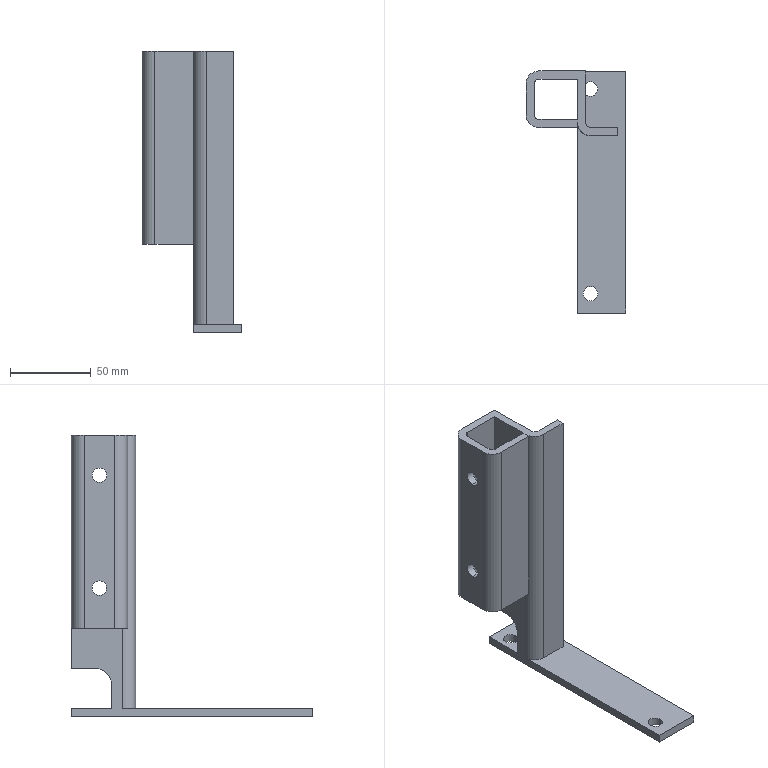Part | SolidWorks | features BaseBody 1 | 1 solid | 40 faces | box 62 x 150 x 175 mm | volume 117135 mm3 | plane 21 | cylinder 19 | commonest cylinder face diameters 9 x12 6 x3 16 x3 20 x1
STEP:
#1=CARTESIAN_POINT('',(0.,-17.5,149.5));
#2=VERTEX_POINT('',#1);
#3=CARTESIAN_POINT('',(0.,-17.5,140.5));
#4=VERTEX_POINT('',#3);
#5=CARTESIAN_POINT('',(0.,-17.5,145.));
#6=DIRECTION('',(1.,0.,0.));
#7=DIRECTION('',(0.,0.,-1.));
#8=AXIS2_PLACEMENT_3D('',#5,#6,#7);
#9=CIRCLE('',#8,4.5);
#10=EDGE_CURVE('',#2,#4,#9,.T.);
#11=ORIENTED_EDGE('',*,*,#10,.F.);
#12=CARTESIAN_POINT('',(5.,-17.5,149.5));
#13=VERTEX_POINT('',#12);
#14=CARTESIAN_POINT('',(0.,-17.5,149.5));
#15=DIRECTION('',(1.,0.,0.));
#16=VECTOR('',#15,1000.);
#17=LINE('',#14,#16);
#18=EDGE_CURVE('',#2,#13,#17,.T.);
#19=ORIENTED_EDGE('',*,*,#18,.T.);
#20=CARTESIAN_POINT('',(5.,-17.5,140.5));
#21=VERTEX_POINT('',#20);
#22=CARTESIAN_POINT('',(5.,-17.5,145.));
#23=DIRECTION('',(-1.,0.,0.));
#24=DIRECTION('',(0.,0.,-1.));
#25=AXIS2_PLACEMENT_3D('',#22,#23,#24);
#26=CIRCLE('',#25,4.5);
#27=EDGE_CURVE('',#21,#13,#26,.T.);
#28=ORIENTED_EDGE('',*,*,#27,.F.);
#29=CARTESIAN_POINT('',(0.,-17.5,140.5));
#30=DIRECTION('',(1.,0.,0.));
#31=VECTOR('',#30,1000.);
#32=LINE('',#29,#31);
#33=EDGE_CURVE('',#4,#21,#32,.T.);
#34=ORIENTED_EDGE('',*,*,#33,.F.);
#35=EDGE_LOOP('',(#11,#19,#28,#34));
#36=FACE_OUTER_BOUND('',#35,.T.);
#37=CARTESIAN_POINT('',(0.,-17.5,145.));
#38=DIRECTION('',(1.,0.,0.));
#39=DIRECTION('',(0.,0.,-1.));
#40=AXIS2_PLACEMENT_3D('',#37,#38,#39);
#41=CYLINDRICAL_SURFACE('',#40,4.5);
#42=ADVANCED_FACE('',(#36),#41,.F.);
#43=CARTESIAN_POINT('',(0.,-17.5,79.5));
#44=VERTEX_POINT('',#43);
#45=CARTESIAN_POINT('',(0.,-17.5,70.5));
#46=VERTEX_POINT('',#45);
#47=CARTESIAN_POINT('',(0.,-17.5,75.));
#48=DIRECTION('',(1.,0.,0.));
#49=DIRECTION('',(0.,0.,-1.));
#50=AXIS2_PLACEMENT_3D('',#47,#48,#49);
#51=CIRCLE('',#50,4.5);
#52=EDGE_CURVE('',#44,#46,#51,.T.);
#53=ORIENTED_EDGE('',*,*,#52,.F.);
#54=CARTESIAN_POINT('',(5.,-17.5,79.5));
#55=VERTEX_POINT('',#54);
#56=CARTESIAN_POINT('',(0.,-17.5,79.5));
#57=DIRECTION('',(1.,0.,0.));
#58=VECTOR('',#57,1000.);
#59=LINE('',#56,#58);
#60=EDGE_CURVE('',#44,#55,#59,.T.);
#61=ORIENTED_EDGE('',*,*,#60,.T.);
#62=CARTESIAN_POINT('',(5.,-17.5,70.5));
#63=VERTEX_POINT('',#62);
#64=CARTESIAN_POINT('',(5.,-17.5,75.));
#65=DIRECTION('',(-1.,0.,0.));
#66=DIRECTION('',(0.,0.,-1.));
#67=AXIS2_PLACEMENT_3D('',#64,#65,#66);
#68=CIRCLE('',#67,4.5);
#69=EDGE_CURVE('',#63,#55,#68,.T.);
#70=ORIENTED_EDGE('',*,*,#69,.F.);
#71=CARTESIAN_POINT('',(0.,-17.5,70.5));
#72=DIRECTION('',(1.,0.,0.));
#73=VECTOR('',#72,1000.);
#74=LINE('',#71,#73);
#75=EDGE_CURVE('',#46,#63,#74,.T.);
#76=ORIENTED_EDGE('',*,*,#75,.F.);
#77=EDGE_LOOP('',(#53,#61,#70,#76));
#78=FACE_OUTER_BOUND('',#77,.T.);
#79=CARTESIAN_POINT('',(0.,-17.5,75.));
#80=DIRECTION('',(1.,0.,0.));
#81=DIRECTION('',(0.,0.,-1.));
#82=AXIS2_PLACEMENT_3D('',#79,#80,#81);
#83=CYLINDRICAL_SURFACE('',#82,4.5);
#84=ADVANCED_FACE('',(#78),#83,.F.);
#85=CARTESIAN_POINT('',(3.5,-11.,-5.));
#86=VERTEX_POINT('',#85);
#87=CARTESIAN_POINT('',(12.5,-11.,-5.));
#88=VERTEX_POINT('',#87);
#89=CARTESIAN_POINT('',(8.,-11.,-5.));
#90=DIRECTION('',(0.,0.,1.));
#91=DIRECTION('',(1.,0.,0.));
#92=AXIS2_PLACEMENT_3D('',#89,#90,#91);
#93=CIRCLE('',#92,4.5);
#94=EDGE_CURVE('',#86,#88,#93,.T.);
#95=ORIENTED_EDGE('',*,*,#94,.F.);
#96=CARTESIAN_POINT('',(3.5,-11.,0.));
#97=VERTEX_POINT('',#96);
#98=CARTESIAN_POINT('',(3.5,-11.,-5.));
#99=DIRECTION('',(0.,0.,1.));
#100=VECTOR('',#99,1000.);
#101=LINE('',#98,#100);
#102=EDGE_CURVE('',#86,#97,#101,.T.);
#103=ORIENTED_EDGE('',*,*,#102,.T.);
#104=CARTESIAN_POINT('',(12.5,-11.,0.));
#105=VERTEX_POINT('',#104);
#106=CARTESIAN_POINT('',(8.,-11.,0.));
#107=DIRECTION('',(0.,0.,-1.));
#108=DIRECTION('',(1.,0.,0.));
#109=AXIS2_PLACEMENT_3D('',#106,#107,#108);
#110=CIRCLE('',#109,4.5);
#111=EDGE_CURVE('',#105,#97,#110,.T.);
#112=ORIENTED_EDGE('',*,*,#111,.F.);
#113=CARTESIAN_POINT('',(12.5,-11.,-5.));
#114=DIRECTION('',(0.,0.,1.));
#115=VECTOR('',#114,1000.);
#116=LINE('',#113,#115);
#117=EDGE_CURVE('',#88,#105,#116,.T.);
#118=ORIENTED_EDGE('',*,*,#117,.F.);
#119=EDGE_LOOP('',(#95,#103,#112,#118));
#120=FACE_OUTER_BOUND('',#119,.T.);
#121=CARTESIAN_POINT('',(8.,-11.,-5.));
#122=DIRECTION('',(0.,0.,1.));
#123=DIRECTION('',(1.,0.,0.));
#124=AXIS2_PLACEMENT_3D('',#121,#122,#123);
#125=CYLINDRICAL_SURFACE('',#124,4.5);
#126=ADVANCED_FACE('',(#120),#125,.F.);
#127=CARTESIAN_POINT('',(3.5,-138.,-5.));
#128=VERTEX_POINT('',#127);
#129=CARTESIAN_POINT('',(12.5,-138.,-5.));
#130=VERTEX_POINT('',#129);
#131=CARTESIAN_POINT('',(8.,-138.,-5.));
#132=DIRECTION('',(0.,0.,1.));
#133=DIRECTION('',(1.,0.,0.));
#134=AXIS2_PLACEMENT_3D('',#131,#132,#133);
#135=CIRCLE('',#134,4.5);
#136=EDGE_CURVE('',#128,#130,#135,.T.);
#137=ORIENTED_EDGE('',*,*,#136,.F.);
#138=CARTESIAN_POINT('',(3.5,-138.,0.));
#139=VERTEX_POINT('',#138);
#140=CARTESIAN_POINT('',(3.5,-138.,-5.));
#141=DIRECTION('',(0.,0.,1.));
#142=VECTOR('',#141,1000.);
#143=LINE('',#140,#142);
#144=EDGE_CURVE('',#128,#139,#143,.T.);
#145=ORIENTED_EDGE('',*,*,#144,.T.);
#146=CARTESIAN_POINT('',(12.5,-138.,0.));
#147=VERTEX_POINT('',#146);
#148=CARTESIAN_POINT('',(8.,-138.,0.));
#149=DIRECTION('',(0.,0.,-1.));
#150=DIRECTION('',(1.,0.,0.));
#151=AXIS2_PLACEMENT_3D('',#148,#149,#150);
#152=CIRCLE('',#151,4.5);
#153=EDGE_CURVE('',#147,#139,#152,.T.);
#154=ORIENTED_EDGE('',*,*,#153,.F.);
#155=CARTESIAN_POINT('',(12.5,-138.,-5.));
#156=DIRECTION('',(0.,0.,1.));
#157=VECTOR('',#156,1000.);
#158=LINE('',#155,#157);
#159=EDGE_CURVE('',#130,#147,#158,.T.);
#160=ORIENTED_EDGE('',*,*,#159,.F.);
#161=EDGE_LOOP('',(#137,#145,#154,#160));
#162=FACE_OUTER_BOUND('',#161,.T.);
#163=CARTESIAN_POINT('',(8.,-138.,-5.));
#164=DIRECTION('',(0.,0.,1.));
#165=DIRECTION('',(1.,0.,0.));
#166=AXIS2_PLACEMENT_3D('',#163,#164,#165);
#167=CYLINDRICAL_SURFACE('',#166,4.5);
#168=ADVANCED_FACE('',(#162),#167,.F.);
#169=CARTESIAN_POINT('',(-27.,-17.5,140.5));
#170=VERTEX_POINT('',#169);
#171=CARTESIAN_POINT('',(-27.,-17.5,149.5));
#172=VERTEX_POINT('',#171);
#173=CARTESIAN_POINT('',(-27.,-17.5,145.));
#174=DIRECTION('',(-1.,0.,0.));
#175=DIRECTION('',(0.,0.,1.));
#176=AXIS2_PLACEMENT_3D('',#173,#174,#175);
#177=CIRCLE('',#176,4.5);
#178=EDGE_CURVE('',#170,#172,#177,.T.);
#179=ORIENTED_EDGE('',*,*,#178,.F.);
#180=CARTESIAN_POINT('',(-32.,-17.5,140.5));
#181=VERTEX_POINT('',#180);
#182=CARTESIAN_POINT('',(-27.,-17.5,140.5));
#183=DIRECTION('',(-1.,0.,0.));
#184=VECTOR('',#183,1000.);
#185=LINE('',#182,#184);
#186=EDGE_CURVE('',#170,#181,#185,.T.);
#187=ORIENTED_EDGE('',*,*,#186,.T.);
#188=CARTESIAN_POINT('',(-32.,-17.5,149.5));
#189=VERTEX_POINT('',#188);
#190=CARTESIAN_POINT('',(-32.,-17.5,145.));
#191=DIRECTION('',(-1.,0.,0.));
#192=DIRECTION('',(0.,0.,1.));
#193=AXIS2_PLACEMENT_3D('',#190,#191,#192);
#194=CIRCLE('',#193,4.5);
#195=EDGE_CURVE('',#181,#189,#194,.T.);
#196=ORIENTED_EDGE('',*,*,#195,.T.);
#197=CARTESIAN_POINT('',(-27.,-17.5,149.5));
#198=DIRECTION('',(-1.,0.,0.));
#199=VECTOR('',#198,1000.);
#200=LINE('',#197,#199);
#201=EDGE_CURVE('',#172,#189,#200,.T.);
#202=ORIENTED_EDGE('',*,*,#201,.F.);
#203=EDGE_LOOP('',(#179,#187,#196,#202));
#204=FACE_OUTER_BOUND('',#203,.T.);
#205=CARTESIAN_POINT('',(-27.,-17.5,145.));
#206=DIRECTION('',(-1.,0.,0.));
#207=DIRECTION('',(0.,0.,1.));
#208=AXIS2_PLACEMENT_3D('',#205,#206,#207);
#209=CYLINDRICAL_SURFACE('',#208,4.5);
#210=ADVANCED_FACE('',(#204),#209,.F.);
#211=CARTESIAN_POINT('',(-27.,-17.5,70.5));
#212=VERTEX_POINT('',#211);
#213=CARTESIAN_POINT('',(-27.,-17.5,79.5));
#214=VERTEX_POINT('',#213);
#215=CARTESIAN_POINT('',(-27.,-17.5,75.));
#216=DIRECTION('',(-1.,0.,0.));
#217=DIRECTION('',(0.,0.,1.));
#218=AXIS2_PLACEMENT_3D('',#215,#216,#217);
#219=CIRCLE('',#218,4.5);
#220=EDGE_CURVE('',#212,#214,#219,.T.);
#221=ORIENTED_EDGE('',*,*,#220,.F.);
#222=CARTESIAN_POINT('',(-32.,-17.5,70.5));
#223=VERTEX_POINT('',#222);
#224=CARTESIAN_POINT('',(-27.,-17.5,70.5));
#225=DIRECTION('',(-1.,0.,0.));
#226=VECTOR('',#225,1000.);
#227=LINE('',#224,#226);
#228=EDGE_CURVE('',#212,#223,#227,.T.);
#229=ORIENTED_EDGE('',*,*,#228,.T.);
#230=CARTESIAN_POINT('',(-32.,-17.5,79.5));
#231=VERTEX_POINT('',#230);
#232=CARTESIAN_POINT('',(-32.,-17.5,75.));
#233=DIRECTION('',(-1.,0.,0.));
#234=DIRECTION('',(0.,0.,1.));
#235=AXIS2_PLACEMENT_3D('',#232,#233,#234);
#236=CIRCLE('',#235,4.5);
#237=EDGE_CURVE('',#223,#231,#236,.T.);
#238=ORIENTED_EDGE('',*,*,#237,.T.);
#239=CARTESIAN_POINT('',(-27.,-17.5,79.5));
#240=DIRECTION('',(-1.,0.,0.));
#241=VECTOR('',#240,1000.);
#242=LINE('',#239,#241);
#243=EDGE_CURVE('',#214,#231,#242,.T.);
#244=ORIENTED_EDGE('',*,*,#243,.F.);
#245=EDGE_LOOP('',(#221,#229,#238,#244));
#246=FACE_OUTER_BOUND('',#245,.T.);
#247=CARTESIAN_POINT('',(-27.,-17.5,75.));
#248=DIRECTION('',(-1.,0.,0.));
#249=DIRECTION('',(0.,0.,1.));
#250=AXIS2_PLACEMENT_3D('',#247,#248,#249);
#251=CYLINDRICAL_SURFACE('',#250,4.5);
#252=ADVANCED_FACE('',(#246),#251,.F.);
#253=ORIENTED_EDGE('',*,*,#27,.T.);
#254=CARTESIAN_POINT('',(5.,-17.5,145.));
#255=DIRECTION('',(-1.,0.,0.));
#256=DIRECTION('',(0.,0.,-1.));
#257=AXIS2_PLACEMENT_3D('',#254,#255,#256);
#258=CIRCLE('',#257,4.5);
#259=EDGE_CURVE('',#13,#21,#258,.T.);
#260=ORIENTED_EDGE('',*,*,#259,.T.);
#261=EDGE_LOOP('',(#253,#260));
#262=FACE_BOUND('',#261,.T.);
#263=ORIENTED_EDGE('',*,*,#69,.T.);
#264=CARTESIAN_POINT('',(5.,-17.5,75.));
#265=DIRECTION('',(-1.,0.,0.));
#266=DIRECTION('',(0.,0.,-1.));
#267=AXIS2_PLACEMENT_3D('',#264,#265,#266);
#268=CIRCLE('',#267,4.5);
#269=EDGE_CURVE('',#55,#63,#268,.T.);
#270=ORIENTED_EDGE('',*,*,#269,.T.);
#271=EDGE_LOOP('',(#263,#270));
#272=FACE_BOUND('',#271,.T.);
#273=CARTESIAN_POINT('',(5.,0.,170.));
#274=VERTEX_POINT('',#273);
#275=CARTESIAN_POINT('',(5.,-32.,170.));
#276=VERTEX_POINT('',#275);
#277=CARTESIAN_POINT('',(5.,-16.,170.));
#278=DIRECTION('',(0.,-1.,0.));
#279=VECTOR('',#278,1000.);
#280=LINE('',#277,#279);
#281=EDGE_CURVE('',#274,#276,#280,.T.);
#282=ORIENTED_EDGE('',*,*,#281,.T.);
#283=CARTESIAN_POINT('',(5.,-32.,0.));
#284=VERTEX_POINT('',#283);
#285=CARTESIAN_POINT('',(5.,-32.,85.));
#286=DIRECTION('',(0.,0.,-1.));
#287=VECTOR('',#286,1000.);
#288=LINE('',#285,#287);
#289=EDGE_CURVE('',#276,#284,#288,.T.);
#290=ORIENTED_EDGE('',*,*,#289,.T.);
#291=CARTESIAN_POINT('',(5.,-25.,0.));
#292=VERTEX_POINT('',#291);
#293=CARTESIAN_POINT('',(5.,-16.,0.));
#294=DIRECTION('',(0.,1.,0.));
#295=VECTOR('',#294,1000.);
#296=LINE('',#293,#295);
#297=EDGE_CURVE('',#284,#292,#296,.T.);
#298=ORIENTED_EDGE('',*,*,#297,.T.);
#299=CARTESIAN_POINT('',(5.,-25.,15.));
#300=VERTEX_POINT('',#299);
#301=CARTESIAN_POINT('',(5.,-25.,85.));
#302=DIRECTION('',(0.,0.,1.));
#303=VECTOR('',#302,1000.);
#304=LINE('',#301,#303);
#305=EDGE_CURVE('',#292,#300,#304,.T.);
#306=ORIENTED_EDGE('',*,*,#305,.T.);
#307=CARTESIAN_POINT('',(5.,-15.,25.));
#308=VERTEX_POINT('',#307);
#309=CARTESIAN_POINT('',(5.,-15.,15.));
#310=DIRECTION('',(-1.,0.,0.));
#311=DIRECTION('',(0.,0.,-1.));
#312=AXIS2_PLACEMENT_3D('',#309,#310,#311);
#313=CIRCLE('',#312,10.);
#314=EDGE_CURVE('',#300,#308,#313,.T.);
#315=ORIENTED_EDGE('',*,*,#314,.T.);
#316=CARTESIAN_POINT('',(5.,0.,25.));
#317=VERTEX_POINT('',#316);
#318=CARTESIAN_POINT('',(5.,-16.,25.));
#319=DIRECTION('',(0.,1.,0.));
#320=VECTOR('',#319,1000.);
#321=LINE('',#318,#320);
#322=EDGE_CURVE('',#308,#317,#321,.T.);
#323=ORIENTED_EDGE('',*,*,#322,.T.);
#324=CARTESIAN_POINT('',(5.,0.,85.));
#325=DIRECTION('',(0.,0.,1.));
#326=VECTOR('',#325,1000.);
#327=LINE('',#324,#326);
#328=EDGE_CURVE('',#317,#274,#327,.T.);
#329=ORIENTED_EDGE('',*,*,#328,.T.);
#330=EDGE_LOOP('',(#282,#290,#298,#306,#315,#323,#329));
#331=FACE_OUTER_BOUND('',#330,.T.);
#332=CARTESIAN_POINT('',(5.,-16.,85.));
#333=DIRECTION('',(1.,0.,0.));
#334=DIRECTION('',(0.,0.,-1.));
#335=AXIS2_PLACEMENT_3D('',#332,#333,#334);
#336=PLANE('',#335);
#337=ADVANCED_FACE('',(#262,#272,#331),#336,.T.);
#338=ORIENTED_EDGE('',*,*,#18,.F.);
#339=CARTESIAN_POINT('',(0.,-17.5,145.));
#340=DIRECTION('',(1.,0.,0.));
#341=DIRECTION('',(0.,0.,-1.));
#342=AXIS2_PLACEMENT_3D('',#339,#340,#341);
#343=CIRCLE('',#342,4.5);
#344=EDGE_CURVE('',#4,#2,#343,.T.);
#345=ORIENTED_EDGE('',*,*,#344,.F.);
#346=ORIENTED_EDGE('',*,*,#33,.T.);
#347=ORIENTED_EDGE('',*,*,#259,.F.);
#348=EDGE_LOOP('',(#338,#345,#346,#347));
#349=FACE_OUTER_BOUND('',#348,.T.);
#350=CARTESIAN_POINT('',(0.,-17.5,145.));
#351=DIRECTION('',(1.,0.,0.));
#352=DIRECTION('',(0.,0.,-1.));
#353=AXIS2_PLACEMENT_3D('',#350,#351,#352);
#354=CYLINDRICAL_SURFACE('',#353,4.5);
#355=ADVANCED_FACE('',(#349),#354,.F.);
#356=ORIENTED_EDGE('',*,*,#60,.F.);
#357=CARTESIAN_POINT('',(0.,-17.5,75.));
#358=DIRECTION('',(1.,0.,0.));
#359=DIRECTION('',(0.,0.,-1.));
#360=AXIS2_PLACEMENT_3D('',#357,#358,#359);
#361=CIRCLE('',#360,4.5);
#362=EDGE_CURVE('',#46,#44,#361,.T.);
#363=ORIENTED_EDGE('',*,*,#362,.F.);
#364=ORIENTED_EDGE('',*,*,#75,.T.);
#365=ORIENTED_EDGE('',*,*,#269,.F.);
#366=EDGE_LOOP('',(#356,#363,#364,#365));
#367=FACE_OUTER_BOUND('',#366,.T.);
#368=CARTESIAN_POINT('',(0.,-17.5,75.));
#369=DIRECTION('',(1.,0.,0.));
#370=DIRECTION('',(0.,0.,-1.));
#371=AXIS2_PLACEMENT_3D('',#368,#369,#370);
#372=CYLINDRICAL_SURFACE('',#371,4.5);
#373=ADVANCED_FACE('',(#367),#372,.F.);
#374=CARTESIAN_POINT('',(8.,-35.,170.));
#375=VERTEX_POINT('',#374);
#376=CARTESIAN_POINT('',(8.,-32.,170.));
#377=DIRECTION('',(0.,0.,-1.));
#378=DIRECTION('',(-1.,0.,0.));
#379=AXIS2_PLACEMENT_3D('',#376,#377,#378);
#380=CIRCLE('',#379,3.);
#381=EDGE_CURVE('',#375,#276,#380,.T.);
#382=ORIENTED_EDGE('',*,*,#381,.F.);
#383=CARTESIAN_POINT('',(8.,-35.,0.));
#384=VERTEX_POINT('',#383);
#385=CARTESIAN_POINT('',(8.,-35.,170.));
#386=DIRECTION('',(0.,0.,1.));
#387=VECTOR('',#386,1000.);
#388=LINE('',#385,#387);
#389=EDGE_CURVE('',#384,#375,#388,.T.);
#390=ORIENTED_EDGE('',*,*,#389,.F.);
#391=CARTESIAN_POINT('',(8.,-32.,0.));
#392=DIRECTION('',(0.,0.,1.));
#393=DIRECTION('',(-1.,0.,0.));
#394=AXIS2_PLACEMENT_3D('',#391,#392,#393);
#395=CIRCLE('',#394,3.);
#396=EDGE_CURVE('',#284,#384,#395,.T.);
#397=ORIENTED_EDGE('',*,*,#396,.F.);
#398=ORIENTED_EDGE('',*,*,#289,.F.);
#399=EDGE_LOOP('',(#382,#390,#397,#398));
#400=FACE_OUTER_BOUND('',#399,.T.);
#401=CARTESIAN_POINT('',(8.,-32.,170.));
#402=DIRECTION('',(0.,0.,-1.));
#403=DIRECTION('',(-1.,0.,0.));
#404=AXIS2_PLACEMENT_3D('',#401,#402,#403);
#405=CYLINDRICAL_SURFACE('',#404,3.);
#406=ADVANCED_FACE('',(#400),#405,.F.);
#407=CARTESIAN_POINT('',(-24.,-5.,170.));
#408=VERTEX_POINT('',#407);
#409=CARTESIAN_POINT('',(0.,-5.,170.));
#410=VERTEX_POINT('',#409);
#411=CARTESIAN_POINT('',(12.5,-5.,170.));
#412=DIRECTION('',(1.,0.,0.));
#413=VECTOR('',#412,1000.);
#414=LINE('',#411,#413);
#415=EDGE_CURVE('',#408,#410,#414,.T.);
#416=ORIENTED_EDGE('',*,*,#415,.T.);
#417=CARTESIAN_POINT('',(0.,-30.,170.));
#418=VERTEX_POINT('',#417);
#419=CARTESIAN_POINT('',(0.,-20.,170.));
#420=DIRECTION('',(0.,-1.,0.));
#421=VECTOR('',#420,1000.);
#422=LINE('',#419,#421);
#423=EDGE_CURVE('',#410,#418,#422,.T.);
#424=ORIENTED_EDGE('',*,*,#423,.T.);
#425=CARTESIAN_POINT('',(-24.,-30.,170.));
#426=VERTEX_POINT('',#425);
#427=CARTESIAN_POINT('',(12.5,-30.,170.));
#428=DIRECTION('',(-1.,0.,0.));
#429=VECTOR('',#428,1000.);
#430=LINE('',#427,#429);
#431=EDGE_CURVE('',#418,#426,#430,.T.);
#432=ORIENTED_EDGE('',*,*,#431,.T.);
#433=CARTESIAN_POINT('',(-27.,-27.,170.));
#434=VERTEX_POINT('',#433);
#435=CARTESIAN_POINT('',(-24.,-27.,170.));
#436=DIRECTION('',(0.,0.,-1.));
#437=DIRECTION('',(1.,0.,0.));
#438=AXIS2_PLACEMENT_3D('',#435,#436,#437);
#439=CIRCLE('',#438,3.);
#440=EDGE_CURVE('',#426,#434,#439,.T.);
#441=ORIENTED_EDGE('',*,*,#440,.T.);
#442=CARTESIAN_POINT('',(-27.,-8.,170.));
#443=VERTEX_POINT('',#442);
#444=CARTESIAN_POINT('',(-27.,-20.,170.));
#445=DIRECTION('',(0.,1.,0.));
#446=VECTOR('',#445,1000.);
#447=LINE('',#444,#446);
#448=EDGE_CURVE('',#434,#443,#447,.T.);
#449=ORIENTED_EDGE('',*,*,#448,.T.);
#450=CARTESIAN_POINT('',(-24.,-8.,170.));
#451=DIRECTION('',(0.,0.,-1.));
#452=DIRECTION('',(1.,0.,0.));
#453=AXIS2_PLACEMENT_3D('',#450,#451,#452);
#454=CIRCLE('',#453,3.);
#455=EDGE_CURVE('',#443,#408,#454,.T.);
#456=ORIENTED_EDGE('',*,*,#455,.T.);
#457=EDGE_LOOP('',(#416,#424,#432,#441,#449,#456));
#458=FACE_BOUND('',#457,.T.);
#459=CARTESIAN_POINT('',(0.,-35.,170.));
#460=VERTEX_POINT('',#459);
#461=CARTESIAN_POINT('',(0.,-32.,170.));
#462=VERTEX_POINT('',#461);
#463=CARTESIAN_POINT('',(0.,-20.,170.));
#464=DIRECTION('',(0.,1.,0.));
#465=VECTOR('',#464,1000.);
#466=LINE('',#463,#465);
#467=EDGE_CURVE('',#460,#462,#466,.T.);
#468=ORIENTED_EDGE('',*,*,#467,.T.);
#469=CARTESIAN_POINT('',(8.,-40.,170.));
#470=VERTEX_POINT('',#469);
#471=CARTESIAN_POINT('',(8.,-32.,170.));
#472=DIRECTION('',(0.,0.,1.));
#473=DIRECTION('',(-1.,0.,0.));
#474=AXIS2_PLACEMENT_3D('',#471,#472,#473);
#475=CIRCLE('',#474,8.);
#476=EDGE_CURVE('',#462,#470,#475,.T.);
#477=ORIENTED_EDGE('',*,*,#476,.T.);
#478=CARTESIAN_POINT('',(25.,-40.,170.));
#479=VERTEX_POINT('',#478);
#480=CARTESIAN_POINT('',(12.5,-40.,170.));
#481=DIRECTION('',(1.,0.,0.));
#482=VECTOR('',#481,1000.);
#483=LINE('',#480,#482);
#484=EDGE_CURVE('',#470,#479,#483,.T.);
#485=ORIENTED_EDGE('',*,*,#484,.T.);
#486=CARTESIAN_POINT('',(25.,-35.,170.));
#487=VERTEX_POINT('',#486);
#488=CARTESIAN_POINT('',(25.,-20.,170.));
#489=DIRECTION('',(0.,1.,0.));
#490=VECTOR('',#489,1000.);
#491=LINE('',#488,#490);
#492=EDGE_CURVE('',#479,#487,#491,.T.);
#493=ORIENTED_EDGE('',*,*,#492,.T.);
#494=CARTESIAN_POINT('',(12.5,-35.,170.));
#495=DIRECTION('',(-1.,0.,0.));
#496=VECTOR('',#495,1000.);
#497=LINE('',#494,#496);
#498=EDGE_CURVE('',#487,#375,#497,.T.);
#499=ORIENTED_EDGE('',*,*,#498,.T.);
#500=ORIENTED_EDGE('',*,*,#381,.T.);
#501=ORIENTED_EDGE('',*,*,#281,.F.);
#502=CARTESIAN_POINT('',(-24.,0.,170.));
#503=VERTEX_POINT('',#502);
#504=CARTESIAN_POINT('',(12.5,0.,170.));
#505=DIRECTION('',(-1.,0.,0.));
#506=VECTOR('',#505,1000.);
#507=LINE('',#504,#506);
#508=EDGE_CURVE('',#274,#503,#507,.T.);
#509=ORIENTED_EDGE('',*,*,#508,.T.);
#510=CARTESIAN_POINT('',(-32.,-8.,170.));
#511=VERTEX_POINT('',#510);
#512=CARTESIAN_POINT('',(-24.,-8.,170.));
#513=DIRECTION('',(0.,0.,1.));
#514=DIRECTION('',(1.,0.,0.));
#515=AXIS2_PLACEMENT_3D('',#512,#513,#514);
#516=CIRCLE('',#515,8.);
#517=EDGE_CURVE('',#503,#511,#516,.T.);
#518=ORIENTED_EDGE('',*,*,#517,.T.);
#519=CARTESIAN_POINT('',(-32.,-27.,170.));
#520=VERTEX_POINT('',#519);
#521=CARTESIAN_POINT('',(-32.,-20.,170.));
#522=DIRECTION('',(0.,-1.,0.));
#523=VECTOR('',#522,1000.);
#524=LINE('',#521,#523);
#525=EDGE_CURVE('',#511,#520,#524,.T.);
#526=ORIENTED_EDGE('',*,*,#525,.T.);
#527=CARTESIAN_POINT('',(-24.,-35.,170.));
#528=VERTEX_POINT('',#527);
#529=CARTESIAN_POINT('',(-24.,-27.,170.));
#530=DIRECTION('',(0.,0.,1.));
#531=DIRECTION('',(1.,0.,0.));
#532=AXIS2_PLACEMENT_3D('',#529,#530,#531);
#533=CIRCLE('',#532,8.);
#534=EDGE_CURVE('',#520,#528,#533,.T.);
#535=ORIENTED_EDGE('',*,*,#534,.T.);
#536=CARTESIAN_POINT('',(12.5,-35.,170.));
#537=DIRECTION('',(1.,0.,0.));
#538=VECTOR('',#537,1000.);
#539=LINE('',#536,#538);
#540=EDGE_CURVE('',#528,#460,#539,.T.);
#541=ORIENTED_EDGE('',*,*,#540,.T.);
#542=EDGE_LOOP('',(#468,#477,#485,#493,#499,#500,#501,#509,#518,#526,#535,#541));
#543=FACE_OUTER_BOUND('',#542,.T.);
#544=CARTESIAN_POINT('',(12.5,-20.,170.));
#545=DIRECTION('',(0.,0.,1.));
#546=DIRECTION('',(1.,0.,0.));
#547=AXIS2_PLACEMENT_3D('',#544,#545,#546);
#548=PLANE('',#547);
#549=ADVANCED_FACE('',(#458,#543),#548,.T.);
#550=CARTESIAN_POINT('',(-24.,0.,50.));
#551=VERTEX_POINT('',#550);
#552=CARTESIAN_POINT('',(-24.,0.,97.5));
#553=DIRECTION('',(0.,0.,1.));
#554=VECTOR('',#553,1000.);
#555=LINE('',#552,#554);
#556=EDGE_CURVE('',#551,#503,#555,.T.);
#557=ORIENTED_EDGE('',*,*,#556,.T.);
#558=ORIENTED_EDGE('',*,*,#508,.F.);
#559=ORIENTED_EDGE('',*,*,#328,.F.);
#560=CARTESIAN_POINT('',(0.,0.,25.));
#561=VERTEX_POINT('',#560);
#562=CARTESIAN_POINT('',(2.5,0.,25.));
#563=DIRECTION('',(-1.,0.,0.));
#564=VECTOR('',#563,1000.);
#565=LINE('',#562,#564);
#566=EDGE_CURVE('',#317,#561,#565,.T.);
#567=ORIENTED_EDGE('',*,*,#566,.T.);
#568=CARTESIAN_POINT('',(0.,0.,50.));
#569=VERTEX_POINT('',#568);
#570=CARTESIAN_POINT('',(0.,0.,97.5));
#571=DIRECTION('',(0.,0.,1.));
#572=VECTOR('',#571,1000.);
#573=LINE('',#570,#572);
#574=EDGE_CURVE('',#561,#569,#573,.T.);
#575=ORIENTED_EDGE('',*,*,#574,.T.);
#576=CARTESIAN_POINT('',(2.5,0.,50.));
#577=DIRECTION('',(-1.,0.,0.));
#578=VECTOR('',#577,1000.);
#579=LINE('',#576,#578);
#580=EDGE_CURVE('',#569,#551,#579,.T.);
#581=ORIENTED_EDGE('',*,*,#580,.T.);
#582=EDGE_LOOP('',(#557,#558,#559,#567,#575,#581));
#583=FACE_OUTER_BOUND('',#582,.T.);
#584=CARTESIAN_POINT('',(2.5,0.,97.5));
#585=DIRECTION('',(0.,1.,0.));
#586=DIRECTION('',(0.,0.,1.));
#587=AXIS2_PLACEMENT_3D('',#584,#585,#586);
#588=PLANE('',#587);
#589=ADVANCED_FACE('',(#583),#588,.T.);
#590=CARTESIAN_POINT('',(0.,-15.,25.));
#591=VERTEX_POINT('',#590);
#592=CARTESIAN_POINT('',(0.,-7.5,25.));
#593=DIRECTION('',(0.,-1.,0.));
#594=VECTOR('',#593,1000.);
#595=LINE('',#592,#594);
#596=EDGE_CURVE('',#561,#591,#595,.T.);
#597=ORIENTED_EDGE('',*,*,#596,.F.);
#598=ORIENTED_EDGE('',*,*,#566,.F.);
#599=ORIENTED_EDGE('',*,*,#322,.F.);
#600=CARTESIAN_POINT('',(2.5,-15.,25.));
#601=DIRECTION('',(1.,0.,0.));
#602=VECTOR('',#601,1000.);
#603=LINE('',#600,#602);
#604=EDGE_CURVE('',#591,#308,#603,.T.);
#605=ORIENTED_EDGE('',*,*,#604,.F.);
#606=EDGE_LOOP('',(#597,#598,#599,#605));
#607=FACE_OUTER_BOUND('',#606,.T.);
#608=CARTESIAN_POINT('',(2.5,-7.5,25.));
#609=DIRECTION('',(0.,0.,1.));
#610=DIRECTION('',(1.,0.,0.));
#611=AXIS2_PLACEMENT_3D('',#608,#609,#610);
#612=PLANE('',#611);
#613=ADVANCED_FACE('',(#607),#612,.F.);
#614=ORIENTED_EDGE('',*,*,#604,.T.);
#615=ORIENTED_EDGE('',*,*,#314,.F.);
#616=CARTESIAN_POINT('',(0.,-25.,15.));
#617=VERTEX_POINT('',#616);
#618=CARTESIAN_POINT('',(0.,-25.,15.));
#619=DIRECTION('',(1.,0.,0.));
#620=VECTOR('',#619,1000.);
#621=LINE('',#618,#620);
#622=EDGE_CURVE('',#617,#300,#621,.T.);
#623=ORIENTED_EDGE('',*,*,#622,.F.);
#624=CARTESIAN_POINT('',(0.,-15.,15.));
#625=DIRECTION('',(1.,0.,0.));
#626=DIRECTION('',(0.,0.,-1.));
#627=AXIS2_PLACEMENT_3D('',#624,#625,#626);
#628=CIRCLE('',#627,10.);
#629=EDGE_CURVE('',#591,#617,#628,.T.);
#630=ORIENTED_EDGE('',*,*,#629,.F.);
#631=EDGE_LOOP('',(#614,#615,#623,#630));
#632=FACE_OUTER_BOUND('',#631,.T.);
#633=CARTESIAN_POINT('',(0.,-15.,15.));
#634=DIRECTION('',(1.,0.,0.));
#635=DIRECTION('',(0.,0.,-1.));
#636=AXIS2_PLACEMENT_3D('',#633,#634,#635);
#637=CYLINDRICAL_SURFACE('',#636,10.);
#638=ADVANCED_FACE('',(#632),#637,.F.);
#639=ORIENTED_EDGE('',*,*,#305,.F.);
#640=CARTESIAN_POINT('',(0.,-25.,0.));
#641=VERTEX_POINT('',#640);
#642=CARTESIAN_POINT('',(2.5,-25.,0.));
#643=DIRECTION('',(-1.,0.,0.));
#644=VECTOR('',#643,1000.);
#645=LINE('',#642,#644);
#646=EDGE_CURVE('',#292,#641,#645,.T.);
#647=ORIENTED_EDGE('',*,*,#646,.T.);
#648=CARTESIAN_POINT('',(0.,-25.,7.5));
#649=DIRECTION('',(0.,0.,1.));
#650=VECTOR('',#649,1000.);
#651=LINE('',#648,#650);
#652=EDGE_CURVE('',#641,#617,#651,.T.);
#653=ORIENTED_EDGE('',*,*,#652,.T.);
#654=ORIENTED_EDGE('',*,*,#622,.T.);
#655=EDGE_LOOP('',(#639,#647,#653,#654));
#656=FACE_OUTER_BOUND('',#655,.T.);
#657=CARTESIAN_POINT('',(2.5,-25.,7.5));
#658=DIRECTION('',(0.,1.,0.));
#659=DIRECTION('',(0.,0.,1.));
#660=AXIS2_PLACEMENT_3D('',#657,#658,#659);
#661=PLANE('',#660);
#662=ADVANCED_FACE('',(#656),#661,.T.);
#663=ORIENTED_EDGE('',*,*,#111,.T.);
#664=CARTESIAN_POINT('',(8.,-11.,0.));
#665=DIRECTION('',(0.,0.,-1.));
#666=DIRECTION('',(1.,0.,0.));
#667=AXIS2_PLACEMENT_3D('',#664,#665,#666);
#668=CIRCLE('',#667,4.5);
#669=EDGE_CURVE('',#97,#105,#668,.T.);
#670=ORIENTED_EDGE('',*,*,#669,.T.);
#671=EDGE_LOOP('',(#663,#670));
#672=FACE_BOUND('',#671,.T.);
#673=ORIENTED_EDGE('',*,*,#153,.T.);
#674=CARTESIAN_POINT('',(8.,-138.,0.));
#675=DIRECTION('',(0.,0.,-1.));
#676=DIRECTION('',(1.,0.,0.));
#677=AXIS2_PLACEMENT_3D('',#674,#675,#676);
#678=CIRCLE('',#677,4.5);
#679=EDGE_CURVE('',#139,#147,#678,.T.);
#680=ORIENTED_EDGE('',*,*,#679,.T.);
#681=EDGE_LOOP('',(#673,#680));
#682=FACE_BOUND('',#681,.T.);
#683=CARTESIAN_POINT('',(25.,-35.,0.));
#684=VERTEX_POINT('',#683);
#685=CARTESIAN_POINT('',(25.,-40.,0.));
#686=VERTEX_POINT('',#685);
#687=CARTESIAN_POINT('',(25.,-75.,0.));
#688=DIRECTION('',(0.,-1.,0.));
#689=VECTOR('',#688,1000.);
#690=LINE('',#687,#689);
#691=EDGE_CURVE('',#684,#686,#690,.T.);
#692=ORIENTED_EDGE('',*,*,#691,.T.);
#693=CARTESIAN_POINT('',(8.,-40.,0.));
#694=VERTEX_POINT('',#693);
#695=CARTESIAN_POINT('',(15.,-40.,0.));
#696=DIRECTION('',(-1.,0.,0.));
#697=VECTOR('',#696,1000.);
#698=LINE('',#695,#697);
#699=EDGE_CURVE('',#686,#694,#698,.T.);
#700=ORIENTED_EDGE('',*,*,#699,.T.);
#701=CARTESIAN_POINT('',(0.,-32.,0.));
#702=VERTEX_POINT('',#701);
#703=CARTESIAN_POINT('',(8.,-32.,0.));
#704=DIRECTION('',(0.,0.,-1.));
#705=DIRECTION('',(-1.,0.,0.));
#706=AXIS2_PLACEMENT_3D('',#703,#704,#705);
#707=CIRCLE('',#706,8.);
#708=EDGE_CURVE('',#694,#702,#707,.T.);
#709=ORIENTED_EDGE('',*,*,#708,.T.);
#710=CARTESIAN_POINT('',(0.,-150.,0.));
#711=VERTEX_POINT('',#710);
#712=CARTESIAN_POINT('',(0.,-75.,0.));
#713=DIRECTION('',(0.,-1.,0.));
#714=VECTOR('',#713,1000.);
#715=LINE('',#712,#714);
#716=EDGE_CURVE('',#702,#711,#715,.T.);
#717=ORIENTED_EDGE('',*,*,#716,.T.);
#718=CARTESIAN_POINT('',(30.,-150.,0.));
#719=VERTEX_POINT('',#718);
#720=CARTESIAN_POINT('',(15.,-150.,0.));
#721=DIRECTION('',(1.,0.,0.));
#722=VECTOR('',#721,1000.);
#723=LINE('',#720,#722);
#724=EDGE_CURVE('',#711,#719,#723,.T.);
#725=ORIENTED_EDGE('',*,*,#724,.T.);
#726=CARTESIAN_POINT('',(30.,0.,0.));
#727=VERTEX_POINT('',#726);
#728=CARTESIAN_POINT('',(30.,-75.,0.));
#729=DIRECTION('',(0.,1.,0.));
#730=VECTOR('',#729,1000.);
#731=LINE('',#728,#730);
#732=EDGE_CURVE('',#719,#727,#731,.T.);
#733=ORIENTED_EDGE('',*,*,#732,.T.);
#734=CARTESIAN_POINT('',(0.,0.,0.));
#735=VERTEX_POINT('',#734);
#736=CARTESIAN_POINT('',(15.,0.,0.));
#737=DIRECTION('',(-1.,0.,0.));
#738=VECTOR('',#737,1000.);
#739=LINE('',#736,#738);
#740=EDGE_CURVE('',#727,#735,#739,.T.);
#741=ORIENTED_EDGE('',*,*,#740,.T.);
#742=CARTESIAN_POINT('',(0.,-75.,0.));
#743=DIRECTION('',(0.,-1.,0.));
#744=VECTOR('',#743,1000.);
#745=LINE('',#742,#744);
#746=EDGE_CURVE('',#735,#641,#745,.T.);
#747=ORIENTED_EDGE('',*,*,#746,.T.);
#748=ORIENTED_EDGE('',*,*,#646,.F.);
#749=ORIENTED_EDGE('',*,*,#297,.F.);
#750=ORIENTED_EDGE('',*,*,#396,.T.);
#751=CARTESIAN_POINT('',(15.,-35.,0.));
#752=DIRECTION('',(1.,0.,0.));
#753=VECTOR('',#752,1000.);
#754=LINE('',#751,#753);
#755=EDGE_CURVE('',#384,#684,#754,.T.);
#756=ORIENTED_EDGE('',*,*,#755,.T.);
#757=EDGE_LOOP('',(#692,#700,#709,#717,#725,#733,#741,#747,#748,#749,#750,#756));
#758=FACE_OUTER_BOUND('',#757,.T.);
#759=CARTESIAN_POINT('',(15.,-75.,0.));
#760=DIRECTION('',(0.,0.,1.));
#761=DIRECTION('',(1.,0.,0.));
#762=AXIS2_PLACEMENT_3D('',#759,#760,#761);
#763=PLANE('',#762);
#764=ADVANCED_FACE('',(#672,#682,#758),#763,.T.);
#765=ORIENTED_EDGE('',*,*,#362,.T.);
#766=ORIENTED_EDGE('',*,*,#52,.T.);
#767=EDGE_LOOP('',(#765,#766));
#768=FACE_BOUND('',#767,.T.);
#769=ORIENTED_EDGE('',*,*,#344,.T.);
#770=ORIENTED_EDGE('',*,*,#10,.T.);
#771=EDGE_LOOP('',(#769,#770));
#772=FACE_BOUND('',#771,.T.);
#773=CARTESIAN_POINT('',(0.,-5.,50.));
#774=VERTEX_POINT('',#773);
#775=CARTESIAN_POINT('',(0.,-5.,-2.5));
#776=DIRECTION('',(0.,0.,1.));
#777=VECTOR('',#776,1000.);
#778=LINE('',#775,#777);
#779=EDGE_CURVE('',#774,#410,#778,.T.);
#780=ORIENTED_EDGE('',*,*,#779,.F.);
#781=CARTESIAN_POINT('',(0.,-75.,50.));
#782=DIRECTION('',(0.,-1.,0.));
#783=VECTOR('',#782,1000.);
#784=LINE('',#781,#783);
#785=EDGE_CURVE('',#569,#774,#784,.T.);
#786=ORIENTED_EDGE('',*,*,#785,.F.);
#787=ORIENTED_EDGE('',*,*,#574,.F.);
#788=ORIENTED_EDGE('',*,*,#596,.T.);
#789=ORIENTED_EDGE('',*,*,#629,.T.);
#790=ORIENTED_EDGE('',*,*,#652,.F.);
#791=ORIENTED_EDGE('',*,*,#746,.F.);
#792=CARTESIAN_POINT('',(0.,0.,-5.));
#793=VERTEX_POINT('',#792);
#794=CARTESIAN_POINT('',(0.,0.,-2.5));
#795=DIRECTION('',(0.,0.,1.));
#796=VECTOR('',#795,1000.);
#797=LINE('',#794,#796);
#798=EDGE_CURVE('',#793,#735,#797,.T.);
#799=ORIENTED_EDGE('',*,*,#798,.F.);
#800=CARTESIAN_POINT('',(0.,-150.,-5.));
#801=VERTEX_POINT('',#800);
#802=CARTESIAN_POINT('',(0.,-75.,-5.));
#803=DIRECTION('',(0.,1.,0.));
#804=VECTOR('',#803,1000.);
#805=LINE('',#802,#804);
#806=EDGE_CURVE('',#801,#793,#805,.T.);
#807=ORIENTED_EDGE('',*,*,#806,.F.);
#808=CARTESIAN_POINT('',(0.,-150.,-2.5));
#809=DIRECTION('',(0.,0.,-1.));
#810=VECTOR('',#809,1000.);
#811=LINE('',#808,#810);
#812=EDGE_CURVE('',#711,#801,#811,.T.);
#813=ORIENTED_EDGE('',*,*,#812,.F.);
#814=ORIENTED_EDGE('',*,*,#716,.F.);
#815=CARTESIAN_POINT('',(0.,-32.,50.));
#816=VERTEX_POINT('',#815);
#817=CARTESIAN_POINT('',(0.,-32.,-2.5));
#818=DIRECTION('',(0.,0.,-1.));
#819=VECTOR('',#818,1000.);
#820=LINE('',#817,#819);
#821=EDGE_CURVE('',#816,#702,#820,.T.);
#822=ORIENTED_EDGE('',*,*,#821,.F.);
#823=CARTESIAN_POINT('',(0.,-30.,50.));
#824=VERTEX_POINT('',#823);
#825=CARTESIAN_POINT('',(0.,-75.,50.));
#826=DIRECTION('',(0.,-1.,0.));
#827=VECTOR('',#826,1000.);
#828=LINE('',#825,#827);
#829=EDGE_CURVE('',#824,#816,#828,.T.);
#830=ORIENTED_EDGE('',*,*,#829,.F.);
#831=CARTESIAN_POINT('',(0.,-30.,-2.5));
#832=DIRECTION('',(0.,0.,-1.));
#833=VECTOR('',#832,1000.);
#834=LINE('',#831,#833);
#835=EDGE_CURVE('',#418,#824,#834,.T.);
#836=ORIENTED_EDGE('',*,*,#835,.F.);
#837=ORIENTED_EDGE('',*,*,#423,.F.);
#838=EDGE_LOOP('',(#780,#786,#787,#788,#789,#790,#791,#799,#807,#813,#814,#822,#830,#836,#837));
#839=FACE_OUTER_BOUND('',#838,.T.);
#840=CARTESIAN_POINT('',(0.,-75.,-2.5));
#841=DIRECTION('',(1.,0.,0.));
#842=DIRECTION('',(0.,0.,-1.));
#843=AXIS2_PLACEMENT_3D('',#840,#841,#842);
#844=PLANE('',#843);
#845=ADVANCED_FACE('',(#768,#772,#839),#844,.F.);
#846=CARTESIAN_POINT('',(25.,-35.,85.));
#847=DIRECTION('',(0.,0.,-1.));
#848=VECTOR('',#847,1000.);
#849=LINE('',#846,#848);
#850=EDGE_CURVE('',#487,#684,#849,.T.);
#851=ORIENTED_EDGE('',*,*,#850,.T.);
#852=ORIENTED_EDGE('',*,*,#755,.F.);
#853=ORIENTED_EDGE('',*,*,#389,.T.);
#854=ORIENTED_EDGE('',*,*,#498,.F.);
#855=EDGE_LOOP('',(#851,#852,#853,#854));
#856=FACE_OUTER_BOUND('',#855,.T.);
#857=CARTESIAN_POINT('',(16.5,-35.,85.));
#858=DIRECTION('',(0.,1.,0.));
#859=DIRECTION('',(0.,0.,1.));
#860=AXIS2_PLACEMENT_3D('',#857,#858,#859);
#861=PLANE('',#860);
#862=ADVANCED_FACE('',(#856),#861,.T.);
#863=CARTESIAN_POINT('',(-24.,-5.,50.));
#864=VERTEX_POINT('',#863);
#865=CARTESIAN_POINT('',(-24.,-5.,110.));
#866=DIRECTION('',(0.,0.,1.));
#867=VECTOR('',#866,1000.);
#868=LINE('',#865,#867);
#869=EDGE_CURVE('',#864,#408,#868,.T.);
#870=ORIENTED_EDGE('',*,*,#869,.F.);
#871=CARTESIAN_POINT('',(-12.,-5.,50.));
#872=DIRECTION('',(-1.,0.,0.));
#873=VECTOR('',#872,1000.);
#874=LINE('',#871,#873);
#875=EDGE_CURVE('',#774,#864,#874,.T.);
#876=ORIENTED_EDGE('',*,*,#875,.F.);
#877=ORIENTED_EDGE('',*,*,#779,.T.);
#878=ORIENTED_EDGE('',*,*,#415,.F.);
#879=EDGE_LOOP('',(#870,#876,#877,#878));
#880=FACE_OUTER_BOUND('',#879,.T.);
#881=CARTESIAN_POINT('',(-12.,-5.,110.));
#882=DIRECTION('',(0.,1.,0.));
#883=DIRECTION('',(0.,0.,1.));
#884=AXIS2_PLACEMENT_3D('',#881,#882,#883);
#885=PLANE('',#884);
#886=ADVANCED_FACE('',(#880),#885,.F.);
#887=ORIENTED_EDGE('',*,*,#869,.T.);
#888=ORIENTED_EDGE('',*,*,#455,.F.);
#889=CARTESIAN_POINT('',(-27.,-8.,50.));
#890=VERTEX_POINT('',#889);
#891=CARTESIAN_POINT('',(-27.,-8.,50.));
#892=DIRECTION('',(0.,0.,1.));
#893=VECTOR('',#892,1000.);
#894=LINE('',#891,#893);
#895=EDGE_CURVE('',#890,#443,#894,.T.);
#896=ORIENTED_EDGE('',*,*,#895,.F.);
#897=CARTESIAN_POINT('',(-24.,-8.,50.));
#898=DIRECTION('',(0.,0.,1.));
#899=DIRECTION('',(1.,0.,0.));
#900=AXIS2_PLACEMENT_3D('',#897,#898,#899);
#901=CIRCLE('',#900,3.);
#902=EDGE_CURVE('',#864,#890,#901,.T.);
#903=ORIENTED_EDGE('',*,*,#902,.F.);
#904=EDGE_LOOP('',(#887,#888,#896,#903));
#905=FACE_OUTER_BOUND('',#904,.T.);
#906=CARTESIAN_POINT('',(-24.,-8.,50.));
#907=DIRECTION('',(0.,0.,1.));
#908=DIRECTION('',(1.,0.,0.));
#909=AXIS2_PLACEMENT_3D('',#906,#907,#908);
#910=CYLINDRICAL_SURFACE('',#909,3.);
#911=ADVANCED_FACE('',(#905),#910,.F.);
#912=CARTESIAN_POINT('',(-27.,-17.5,145.));
#913=DIRECTION('',(-1.,0.,0.));
#914=DIRECTION('',(0.,0.,1.));
#915=AXIS2_PLACEMENT_3D('',#912,#913,#914);
#916=CIRCLE('',#915,4.5);
#917=EDGE_CURVE('',#172,#170,#916,.T.);
#918=ORIENTED_EDGE('',*,*,#917,.T.);
#919=ORIENTED_EDGE('',*,*,#178,.T.);
#920=EDGE_LOOP('',(#918,#919));
#921=FACE_BOUND('',#920,.T.);
#922=CARTESIAN_POINT('',(-27.,-17.5,75.));
#923=DIRECTION('',(-1.,0.,0.));
#924=DIRECTION('',(0.,0.,1.));
#925=AXIS2_PLACEMENT_3D('',#922,#923,#924);
#926=CIRCLE('',#925,4.5);
#927=EDGE_CURVE('',#214,#212,#926,.T.);
#928=ORIENTED_EDGE('',*,*,#927,.T.);
#929=ORIENTED_EDGE('',*,*,#220,.T.);
#930=EDGE_LOOP('',(#928,#929));
#931=FACE_BOUND('',#930,.T.);
#932=CARTESIAN_POINT('',(-27.,-27.,50.));
#933=VERTEX_POINT('',#932);
#934=CARTESIAN_POINT('',(-27.,-27.,110.));
#935=DIRECTION('',(0.,0.,-1.));
#936=VECTOR('',#935,1000.);
#937=LINE('',#934,#936);
#938=EDGE_CURVE('',#434,#933,#937,.T.);
#939=ORIENTED_EDGE('',*,*,#938,.T.);
#940=CARTESIAN_POINT('',(-27.,-17.5,50.));
#941=DIRECTION('',(0.,1.,0.));
#942=VECTOR('',#941,1000.);
#943=LINE('',#940,#942);
#944=EDGE_CURVE('',#933,#890,#943,.T.);
#945=ORIENTED_EDGE('',*,*,#944,.T.);
#946=ORIENTED_EDGE('',*,*,#895,.T.);
#947=ORIENTED_EDGE('',*,*,#448,.F.);
#948=EDGE_LOOP('',(#939,#945,#946,#947));
#949=FACE_OUTER_BOUND('',#948,.T.);
#950=CARTESIAN_POINT('',(-27.,-17.5,110.));
#951=DIRECTION('',(1.,0.,0.));
#952=DIRECTION('',(0.,0.,-1.));
#953=AXIS2_PLACEMENT_3D('',#950,#951,#952);
#954=PLANE('',#953);
#955=ADVANCED_FACE('',(#921,#931,#949),#954,.T.);
#956=ORIENTED_EDGE('',*,*,#938,.F.);
#957=ORIENTED_EDGE('',*,*,#440,.F.);
#958=CARTESIAN_POINT('',(-24.,-30.,50.));
#959=VERTEX_POINT('',#958);
#960=CARTESIAN_POINT('',(-24.,-30.,50.));
#961=DIRECTION('',(0.,0.,1.));
#962=VECTOR('',#961,1000.);
#963=LINE('',#960,#962);
#964=EDGE_CURVE('',#959,#426,#963,.T.);
#965=ORIENTED_EDGE('',*,*,#964,.F.);
#966=CARTESIAN_POINT('',(-24.,-27.,50.));
#967=DIRECTION('',(0.,0.,1.));
#968=DIRECTION('',(1.,0.,0.));
#969=AXIS2_PLACEMENT_3D('',#966,#967,#968);
#970=CIRCLE('',#969,3.);
#971=EDGE_CURVE('',#933,#959,#970,.T.);
#972=ORIENTED_EDGE('',*,*,#971,.F.);
#973=EDGE_LOOP('',(#956,#957,#965,#972));
#974=FACE_OUTER_BOUND('',#973,.T.);
#975=CARTESIAN_POINT('',(-24.,-27.,50.));
#976=DIRECTION('',(0.,0.,1.));
#977=DIRECTION('',(1.,0.,0.));
#978=AXIS2_PLACEMENT_3D('',#975,#976,#977);
#979=CYLINDRICAL_SURFACE('',#978,3.);
#980=ADVANCED_FACE('',(#974),#979,.F.);
#981=ORIENTED_EDGE('',*,*,#431,.F.);
#982=ORIENTED_EDGE('',*,*,#835,.T.);
#983=CARTESIAN_POINT('',(-12.,-30.,50.));
#984=DIRECTION('',(-1.,0.,0.));
#985=VECTOR('',#984,1000.);
#986=LINE('',#983,#985);
#987=EDGE_CURVE('',#824,#959,#986,.T.);
#988=ORIENTED_EDGE('',*,*,#987,.T.);
#989=ORIENTED_EDGE('',*,*,#964,.T.);
#990=EDGE_LOOP('',(#981,#982,#988,#989));
#991=FACE_OUTER_BOUND('',#990,.T.);
#992=CARTESIAN_POINT('',(-12.,-30.,110.));
#993=DIRECTION('',(0.,1.,0.));
#994=DIRECTION('',(0.,0.,1.));
#995=AXIS2_PLACEMENT_3D('',#992,#993,#994);
#996=PLANE('',#995);
#997=ADVANCED_FACE('',(#991),#996,.T.);
#998=ORIENTED_EDGE('',*,*,#476,.F.);
#999=CARTESIAN_POINT('',(0.,-32.,170.));
#1000=DIRECTION('',(0.,0.,-1.));
#1001=VECTOR('',#1000,1000.);
#1002=LINE('',#999,#1001);
#1003=EDGE_CURVE('',#462,#816,#1002,.T.);
#1004=ORIENTED_EDGE('',*,*,#1003,.T.);
#1005=ORIENTED_EDGE('',*,*,#821,.T.);
#1006=ORIENTED_EDGE('',*,*,#708,.F.);
#1007=CARTESIAN_POINT('',(8.,-40.,170.));
#1008=DIRECTION('',(0.,0.,1.));
#1009=VECTOR('',#1008,1000.);
#1010=LINE('',#1007,#1009);
#1011=EDGE_CURVE('',#694,#470,#1010,.T.);
#1012=ORIENTED_EDGE('',*,*,#1011,.T.);
#1013=EDGE_LOOP('',(#998,#1004,#1005,#1006,#1012));
#1014=FACE_OUTER_BOUND('',#1013,.T.);
#1015=CARTESIAN_POINT('',(8.,-32.,170.));
#1016=DIRECTION('',(0.,0.,-1.));
#1017=DIRECTION('',(-1.,0.,0.));
#1018=AXIS2_PLACEMENT_3D('',#1015,#1016,#1017);
#1019=CYLINDRICAL_SURFACE('',#1018,8.);
#1020=ADVANCED_FACE('',(#1014),#1019,.T.);
#1021=CARTESIAN_POINT('',(0.,-35.,50.));
#1022=VERTEX_POINT('',#1021);
#1023=CARTESIAN_POINT('',(0.,-32.5,50.));
#1024=DIRECTION('',(0.,1.,0.));
#1025=VECTOR('',#1024,1000.);
#1026=LINE('',#1023,#1025);
#1027=EDGE_CURVE('',#1022,#816,#1026,.T.);
#1028=ORIENTED_EDGE('',*,*,#1027,.T.);
#1029=ORIENTED_EDGE('',*,*,#1003,.F.);
#1030=ORIENTED_EDGE('',*,*,#467,.F.);
#1031=CARTESIAN_POINT('',(0.,-35.,110.));
#1032=DIRECTION('',(0.,0.,-1.));
#1033=VECTOR('',#1032,1000.);
#1034=LINE('',#1031,#1033);
#1035=EDGE_CURVE('',#460,#1022,#1034,.T.);
#1036=ORIENTED_EDGE('',*,*,#1035,.T.);
#1037=EDGE_LOOP('',(#1028,#1029,#1030,#1036));
#1038=FACE_OUTER_BOUND('',#1037,.T.);
#1039=CARTESIAN_POINT('',(0.,-32.5,110.));
#1040=DIRECTION('',(1.,0.,0.));
#1041=DIRECTION('',(0.,0.,-1.));
#1042=AXIS2_PLACEMENT_3D('',#1039,#1040,#1041);
#1043=PLANE('',#1042);
#1044=ADVANCED_FACE('',(#1038),#1043,.T.);
#1045=ORIENTED_EDGE('',*,*,#540,.F.);
#1046=CARTESIAN_POINT('',(-24.,-35.,50.));
#1047=VERTEX_POINT('',#1046);
#1048=CARTESIAN_POINT('',(-24.,-35.,110.));
#1049=DIRECTION('',(0.,0.,1.));
#1050=VECTOR('',#1049,1000.);
#1051=LINE('',#1048,#1050);
#1052=EDGE_CURVE('',#1047,#528,#1051,.T.);
#1053=ORIENTED_EDGE('',*,*,#1052,.F.);
#1054=CARTESIAN_POINT('',(-12.,-35.,50.));
#1055=DIRECTION('',(-1.,0.,0.));
#1056=VECTOR('',#1055,1000.);
#1057=LINE('',#1054,#1056);
#1058=EDGE_CURVE('',#1022,#1047,#1057,.T.);
#1059=ORIENTED_EDGE('',*,*,#1058,.F.);
#1060=ORIENTED_EDGE('',*,*,#1035,.F.);
#1061=EDGE_LOOP('',(#1045,#1053,#1059,#1060));
#1062=FACE_OUTER_BOUND('',#1061,.T.);
#1063=CARTESIAN_POINT('',(-12.,-35.,110.));
#1064=DIRECTION('',(0.,1.,0.));
#1065=DIRECTION('',(0.,0.,1.));
#1066=AXIS2_PLACEMENT_3D('',#1063,#1064,#1065);
#1067=PLANE('',#1066);
#1068=ADVANCED_FACE('',(#1062),#1067,.F.);
#1069=ORIENTED_EDGE('',*,*,#534,.F.);
#1070=CARTESIAN_POINT('',(-32.,-27.,50.));
#1071=VERTEX_POINT('',#1070);
#1072=CARTESIAN_POINT('',(-32.,-27.,50.));
#1073=DIRECTION('',(0.,0.,-1.));
#1074=VECTOR('',#1073,1000.);
#1075=LINE('',#1072,#1074);
#1076=EDGE_CURVE('',#520,#1071,#1075,.T.);
#1077=ORIENTED_EDGE('',*,*,#1076,.T.);
#1078=CARTESIAN_POINT('',(-24.,-27.,50.));
#1079=DIRECTION('',(0.,0.,1.));
#1080=DIRECTION('',(1.,0.,0.));
#1081=AXIS2_PLACEMENT_3D('',#1078,#1079,#1080);
#1082=CIRCLE('',#1081,8.);
#1083=EDGE_CURVE('',#1071,#1047,#1082,.T.);
#1084=ORIENTED_EDGE('',*,*,#1083,.T.);
#1085=ORIENTED_EDGE('',*,*,#1052,.T.);
#1086=EDGE_LOOP('',(#1069,#1077,#1084,#1085));
#1087=FACE_OUTER_BOUND('',#1086,.T.);
#1088=CARTESIAN_POINT('',(-24.,-27.,50.));
#1089=DIRECTION('',(0.,0.,1.));
#1090=DIRECTION('',(1.,0.,0.));
#1091=AXIS2_PLACEMENT_3D('',#1088,#1089,#1090);
#1092=CYLINDRICAL_SURFACE('',#1091,8.);
#1093=ADVANCED_FACE('',(#1087),#1092,.T.);
#1094=CARTESIAN_POINT('',(-32.,-17.5,145.));
#1095=DIRECTION('',(-1.,0.,0.));
#1096=DIRECTION('',(0.,0.,1.));
#1097=AXIS2_PLACEMENT_3D('',#1094,#1095,#1096);
#1098=CIRCLE('',#1097,4.5);
#1099=EDGE_CURVE('',#189,#181,#1098,.T.);
#1100=ORIENTED_EDGE('',*,*,#1099,.F.);
#1101=ORIENTED_EDGE('',*,*,#195,.F.);
#1102=EDGE_LOOP('',(#1100,#1101));
#1103=FACE_BOUND('',#1102,.T.);
#1104=CARTESIAN_POINT('',(-32.,-17.5,75.));
#1105=DIRECTION('',(-1.,0.,0.));
#1106=DIRECTION('',(0.,0.,1.));
#1107=AXIS2_PLACEMENT_3D('',#1104,#1105,#1106);
#1108=CIRCLE('',#1107,4.5);
#1109=EDGE_CURVE('',#231,#223,#1108,.T.);
#1110=ORIENTED_EDGE('',*,*,#1109,.F.);
#1111=ORIENTED_EDGE('',*,*,#237,.F.);
#1112=EDGE_LOOP('',(#1110,#1111));
#1113=FACE_BOUND('',#1112,.T.);
#1114=ORIENTED_EDGE('',*,*,#525,.F.);
#1115=CARTESIAN_POINT('',(-32.,-8.,50.));
#1116=VERTEX_POINT('',#1115);
#1117=CARTESIAN_POINT('',(-32.,-8.,110.));
#1118=DIRECTION('',(0.,0.,1.));
#1119=VECTOR('',#1118,1000.);
#1120=LINE('',#1117,#1119);
#1121=EDGE_CURVE('',#1116,#511,#1120,.T.);
#1122=ORIENTED_EDGE('',*,*,#1121,.F.);
#1123=CARTESIAN_POINT('',(-32.,-17.5,50.));
#1124=DIRECTION('',(0.,1.,0.));
#1125=VECTOR('',#1124,1000.);
#1126=LINE('',#1123,#1125);
#1127=EDGE_CURVE('',#1071,#1116,#1126,.T.);
#1128=ORIENTED_EDGE('',*,*,#1127,.F.);
#1129=ORIENTED_EDGE('',*,*,#1076,.F.);
#1130=EDGE_LOOP('',(#1114,#1122,#1128,#1129));
#1131=FACE_OUTER_BOUND('',#1130,.T.);
#1132=CARTESIAN_POINT('',(-32.,-17.5,110.));
#1133=DIRECTION('',(1.,0.,0.));
#1134=DIRECTION('',(0.,0.,-1.));
#1135=AXIS2_PLACEMENT_3D('',#1132,#1133,#1134);
#1136=PLANE('',#1135);
#1137=ADVANCED_FACE('',(#1103,#1113,#1131),#1136,.F.);
#1138=ORIENTED_EDGE('',*,*,#517,.F.);
#1139=ORIENTED_EDGE('',*,*,#556,.F.);
#1140=CARTESIAN_POINT('',(-24.,-8.,50.));
#1141=DIRECTION('',(0.,0.,1.));
#1142=DIRECTION('',(1.,0.,0.));
#1143=AXIS2_PLACEMENT_3D('',#1140,#1141,#1142);
#1144=CIRCLE('',#1143,8.);
#1145=EDGE_CURVE('',#551,#1116,#1144,.T.);
#1146=ORIENTED_EDGE('',*,*,#1145,.T.);
#1147=ORIENTED_EDGE('',*,*,#1121,.T.);
#1148=EDGE_LOOP('',(#1138,#1139,#1146,#1147));
#1149=FACE_OUTER_BOUND('',#1148,.T.);
#1150=CARTESIAN_POINT('',(-24.,-8.,50.));
#1151=DIRECTION('',(0.,0.,1.));
#1152=DIRECTION('',(1.,0.,0.));
#1153=AXIS2_PLACEMENT_3D('',#1150,#1151,#1152);
#1154=CYLINDRICAL_SURFACE('',#1153,8.);
#1155=ADVANCED_FACE('',(#1149),#1154,.T.);
#1156=CARTESIAN_POINT('',(25.,-40.,85.));
#1157=DIRECTION('',(0.,0.,-1.));
#1158=VECTOR('',#1157,1000.);
#1159=LINE('',#1156,#1158);
#1160=EDGE_CURVE('',#479,#686,#1159,.T.);
#1161=ORIENTED_EDGE('',*,*,#1160,.T.);
#1162=ORIENTED_EDGE('',*,*,#691,.F.);
#1163=ORIENTED_EDGE('',*,*,#850,.F.);
#1164=ORIENTED_EDGE('',*,*,#492,.F.);
#1165=EDGE_LOOP('',(#1161,#1162,#1163,#1164));
#1166=FACE_OUTER_BOUND('',#1165,.T.);
#1167=CARTESIAN_POINT('',(25.,-37.5,85.));
#1168=DIRECTION('',(1.,0.,0.));
#1169=DIRECTION('',(0.,0.,-1.));
#1170=AXIS2_PLACEMENT_3D('',#1167,#1168,#1169);
#1171=PLANE('',#1170);
#1172=ADVANCED_FACE('',(#1166),#1171,.T.);
#1173=ORIENTED_EDGE('',*,*,#484,.F.);
#1174=ORIENTED_EDGE('',*,*,#1011,.F.);
#1175=ORIENTED_EDGE('',*,*,#699,.F.);
#1176=ORIENTED_EDGE('',*,*,#1160,.F.);
#1177=EDGE_LOOP('',(#1173,#1174,#1175,#1176));
#1178=FACE_OUTER_BOUND('',#1177,.T.);
#1179=CARTESIAN_POINT('',(16.5,-40.,85.));
#1180=DIRECTION('',(0.,1.,0.));
#1181=DIRECTION('',(0.,0.,1.));
#1182=AXIS2_PLACEMENT_3D('',#1179,#1180,#1181);
#1183=PLANE('',#1182);
#1184=ADVANCED_FACE('',(#1178),#1183,.F.);
#1185=ORIENTED_EDGE('',*,*,#902,.T.);
#1186=ORIENTED_EDGE('',*,*,#944,.F.);
#1187=ORIENTED_EDGE('',*,*,#971,.T.);
#1188=ORIENTED_EDGE('',*,*,#987,.F.);
#1189=ORIENTED_EDGE('',*,*,#829,.T.);
#1190=ORIENTED_EDGE('',*,*,#1027,.F.);
#1191=ORIENTED_EDGE('',*,*,#1058,.T.);
#1192=ORIENTED_EDGE('',*,*,#1083,.F.);
#1193=ORIENTED_EDGE('',*,*,#1127,.T.);
#1194=ORIENTED_EDGE('',*,*,#1145,.F.);
#1195=ORIENTED_EDGE('',*,*,#580,.F.);
#1196=ORIENTED_EDGE('',*,*,#785,.T.);
#1197=ORIENTED_EDGE('',*,*,#875,.T.);
#1198=EDGE_LOOP('',(#1185,#1186,#1187,#1188,#1189,#1190,#1191,#1192,#1193,#1194,#1195,#1196,#1197));
#1199=FACE_OUTER_BOUND('',#1198,.T.);
#1200=CARTESIAN_POINT('',(-16.,-17.5,50.));
#1201=DIRECTION('',(0.,0.,1.));
#1202=DIRECTION('',(1.,0.,0.));
#1203=AXIS2_PLACEMENT_3D('',#1200,#1201,#1202);
#1204=PLANE('',#1203);
#1205=ADVANCED_FACE('',(#1199),#1204,.F.);
#1206=ORIENTED_EDGE('',*,*,#102,.F.);
#1207=CARTESIAN_POINT('',(8.,-11.,-5.));
#1208=DIRECTION('',(0.,0.,1.));
#1209=DIRECTION('',(1.,0.,0.));
#1210=AXIS2_PLACEMENT_3D('',#1207,#1208,#1209);
#1211=CIRCLE('',#1210,4.5);
#1212=EDGE_CURVE('',#88,#86,#1211,.T.);
#1213=ORIENTED_EDGE('',*,*,#1212,.F.);
#1214=ORIENTED_EDGE('',*,*,#117,.T.);
#1215=ORIENTED_EDGE('',*,*,#669,.F.);
#1216=EDGE_LOOP('',(#1206,#1213,#1214,#1215));
#1217=FACE_OUTER_BOUND('',#1216,.T.);
#1218=CARTESIAN_POINT('',(8.,-11.,-5.));
#1219=DIRECTION('',(0.,0.,1.));
#1220=DIRECTION('',(1.,0.,0.));
#1221=AXIS2_PLACEMENT_3D('',#1218,#1219,#1220);
#1222=CYLINDRICAL_SURFACE('',#1221,4.5);
#1223=ADVANCED_FACE('',(#1217),#1222,.F.);
#1224=ORIENTED_EDGE('',*,*,#144,.F.);
#1225=CARTESIAN_POINT('',(8.,-138.,-5.));
#1226=DIRECTION('',(0.,0.,1.));
#1227=DIRECTION('',(1.,0.,0.));
#1228=AXIS2_PLACEMENT_3D('',#1225,#1226,#1227);
#1229=CIRCLE('',#1228,4.5);
#1230=EDGE_CURVE('',#130,#128,#1229,.T.);
#1231=ORIENTED_EDGE('',*,*,#1230,.F.);
#1232=ORIENTED_EDGE('',*,*,#159,.T.);
#1233=ORIENTED_EDGE('',*,*,#679,.F.);
#1234=EDGE_LOOP('',(#1224,#1231,#1232,#1233));
#1235=FACE_OUTER_BOUND('',#1234,.T.);
#1236=CARTESIAN_POINT('',(8.,-138.,-5.));
#1237=DIRECTION('',(0.,0.,1.));
#1238=DIRECTION('',(1.,0.,0.));
#1239=AXIS2_PLACEMENT_3D('',#1236,#1237,#1238);
#1240=CYLINDRICAL_SURFACE('',#1239,4.5);
#1241=ADVANCED_FACE('',(#1235),#1240,.F.);
#1242=ORIENTED_EDGE('',*,*,#798,.T.);
#1243=ORIENTED_EDGE('',*,*,#740,.F.);
#1244=CARTESIAN_POINT('',(30.,0.,-5.));
#1245=VERTEX_POINT('',#1244);
#1246=CARTESIAN_POINT('',(30.,0.,-2.5));
#1247=DIRECTION('',(0.,0.,-1.));
#1248=VECTOR('',#1247,1000.);
#1249=LINE('',#1246,#1248);
#1250=EDGE_CURVE('',#727,#1245,#1249,.T.);
#1251=ORIENTED_EDGE('',*,*,#1250,.T.);
#1252=CARTESIAN_POINT('',(15.,0.,-5.));
#1253=DIRECTION('',(-1.,0.,0.));
#1254=VECTOR('',#1253,1000.);
#1255=LINE('',#1252,#1254);
#1256=EDGE_CURVE('',#1245,#793,#1255,.T.);
#1257=ORIENTED_EDGE('',*,*,#1256,.T.);
#1258=EDGE_LOOP('',(#1242,#1243,#1251,#1257));
#1259=FACE_OUTER_BOUND('',#1258,.T.);
#1260=CARTESIAN_POINT('',(15.,0.,-2.5));
#1261=DIRECTION('',(0.,1.,0.));
#1262=DIRECTION('',(0.,0.,1.));
#1263=AXIS2_PLACEMENT_3D('',#1260,#1261,#1262);
#1264=PLANE('',#1263);
#1265=ADVANCED_FACE('',(#1259),#1264,.T.);
#1266=ORIENTED_EDGE('',*,*,#1250,.F.);
#1267=ORIENTED_EDGE('',*,*,#732,.F.);
#1268=CARTESIAN_POINT('',(30.,-150.,-5.));
#1269=VERTEX_POINT('',#1268);
#1270=CARTESIAN_POINT('',(30.,-150.,-2.5));
#1271=DIRECTION('',(0.,0.,-1.));
#1272=VECTOR('',#1271,1000.);
#1273=LINE('',#1270,#1272);
#1274=EDGE_CURVE('',#719,#1269,#1273,.T.);
#1275=ORIENTED_EDGE('',*,*,#1274,.T.);
#1276=CARTESIAN_POINT('',(30.,-75.,-5.));
#1277=DIRECTION('',(0.,1.,0.));
#1278=VECTOR('',#1277,1000.);
#1279=LINE('',#1276,#1278);
#1280=EDGE_CURVE('',#1269,#1245,#1279,.T.);
#1281=ORIENTED_EDGE('',*,*,#1280,.T.);
#1282=EDGE_LOOP('',(#1266,#1267,#1275,#1281));
#1283=FACE_OUTER_BOUND('',#1282,.T.);
#1284=CARTESIAN_POINT('',(30.,-75.,-2.5));
#1285=DIRECTION('',(1.,0.,0.));
#1286=DIRECTION('',(0.,0.,-1.));
#1287=AXIS2_PLACEMENT_3D('',#1284,#1285,#1286);
#1288=PLANE('',#1287);
#1289=ADVANCED_FACE('',(#1283),#1288,.T.);
#1290=CARTESIAN_POINT('',(15.,-150.,-5.));
#1291=DIRECTION('',(-1.,0.,0.));
#1292=VECTOR('',#1291,1000.);
#1293=LINE('',#1290,#1292);
#1294=EDGE_CURVE('',#1269,#801,#1293,.T.);
#1295=ORIENTED_EDGE('',*,*,#1294,.F.);
#1296=ORIENTED_EDGE('',*,*,#1274,.F.);
#1297=ORIENTED_EDGE('',*,*,#724,.F.);
#1298=ORIENTED_EDGE('',*,*,#812,.T.);
#1299=EDGE_LOOP('',(#1295,#1296,#1297,#1298));
#1300=FACE_OUTER_BOUND('',#1299,.T.);
#1301=CARTESIAN_POINT('',(15.,-150.,-2.5));
#1302=DIRECTION('',(0.,1.,0.));
#1303=DIRECTION('',(0.,0.,1.));
#1304=AXIS2_PLACEMENT_3D('',#1301,#1302,#1303);
#1305=PLANE('',#1304);
#1306=ADVANCED_FACE('',(#1300),#1305,.F.);
#1307=ORIENTED_EDGE('',*,*,#1230,.T.);
#1308=ORIENTED_EDGE('',*,*,#136,.T.);
#1309=EDGE_LOOP('',(#1307,#1308));
#1310=FACE_BOUND('',#1309,.T.);
#1311=ORIENTED_EDGE('',*,*,#1212,.T.);
#1312=ORIENTED_EDGE('',*,*,#94,.T.);
#1313=EDGE_LOOP('',(#1311,#1312));
#1314=FACE_BOUND('',#1313,.T.);
#1315=ORIENTED_EDGE('',*,*,#1256,.F.);
#1316=ORIENTED_EDGE('',*,*,#1280,.F.);
#1317=ORIENTED_EDGE('',*,*,#1294,.T.);
#1318=ORIENTED_EDGE('',*,*,#806,.T.);
#1319=EDGE_LOOP('',(#1315,#1316,#1317,#1318));
#1320=FACE_OUTER_BOUND('',#1319,.T.);
#1321=CARTESIAN_POINT('',(15.,-75.,-5.));
#1322=DIRECTION('',(0.,0.,1.));
#1323=DIRECTION('',(1.,0.,0.));
#1324=AXIS2_PLACEMENT_3D('',#1321,#1322,#1323);
#1325=PLANE('',#1324);
#1326=ADVANCED_FACE('',(#1310,#1314,#1320),#1325,.F.);
#1327=ORIENTED_EDGE('',*,*,#186,.F.);
#1328=ORIENTED_EDGE('',*,*,#917,.F.);
#1329=ORIENTED_EDGE('',*,*,#201,.T.);
#1330=ORIENTED_EDGE('',*,*,#1099,.T.);
#1331=EDGE_LOOP('',(#1327,#1328,#1329,#1330));
#1332=FACE_OUTER_BOUND('',#1331,.T.);
#1333=CARTESIAN_POINT('',(-27.,-17.5,145.));
#1334=DIRECTION('',(-1.,0.,0.));
#1335=DIRECTION('',(0.,0.,1.));
#1336=AXIS2_PLACEMENT_3D('',#1333,#1334,#1335);
#1337=CYLINDRICAL_SURFACE('',#1336,4.5);
#1338=ADVANCED_FACE('',(#1332),#1337,.F.);
#1339=ORIENTED_EDGE('',*,*,#228,.F.);
#1340=ORIENTED_EDGE('',*,*,#927,.F.);
#1341=ORIENTED_EDGE('',*,*,#243,.T.);
#1342=ORIENTED_EDGE('',*,*,#1109,.T.);
#1343=EDGE_LOOP('',(#1339,#1340,#1341,#1342));
#1344=FACE_OUTER_BOUND('',#1343,.T.);
#1345=CARTESIAN_POINT('',(-27.,-17.5,75.));
#1346=DIRECTION('',(-1.,0.,0.));
#1347=DIRECTION('',(0.,0.,1.));
#1348=AXIS2_PLACEMENT_3D('',#1345,#1346,#1347);
#1349=CYLINDRICAL_SURFACE('',#1348,4.5);
#1350=ADVANCED_FACE('',(#1344),#1349,.F.);
#1351=CLOSED_SHELL('',(#42,#84,#126,#168,#210,#252,#337,#355,#373,#406,#549,#589,#613,#638,#662,#764,#845,#862,#886,#911,#955,#980,#997,#1020,#1044,#1068,#1093,#1137,#1155,#1172,#1184,#1205,#1223,#1241,#1265,#1289,#1306,#1326,#1338,#1350));
#1352=MANIFOLD_SOLID_BREP('',#1351);
#1353=CARTESIAN_POINT('',(0.,0.,0.));
#1354=DIRECTION('',(0.,0.,1.));
#1355=DIRECTION('',(1.,0.,0.));
#1356=AXIS2_PLACEMENT_3D('',#1353,#1354,#1355);
#1357=(LENGTH_UNIT()NAMED_UNIT(*)SI_UNIT(.MILLI.,.METRE.));
#1358=UNCERTAINTY_MEASURE_WITH_UNIT(LENGTH_MEASURE(0.00001),#1357,'','');
#1359=(NAMED_UNIT(*)PLANE_ANGLE_UNIT()SI_UNIT($,.RADIAN.));
#1360=(NAMED_UNIT(*)SI_UNIT($,.STERADIAN.)SOLID_ANGLE_UNIT());
#1361=(GEOMETRIC_REPRESENTATION_CONTEXT(3)GLOBAL_UNCERTAINTY_ASSIGNED_CONTEXT((#1358))GLOBAL_UNIT_ASSIGNED_CONTEXT((#1357,#1359,#1360))REPRESENTATION_CONTEXT('',''));
#1362=ADVANCED_BREP_SHAPE_REPRESENTATION('',(#1352,#1356),#1361);